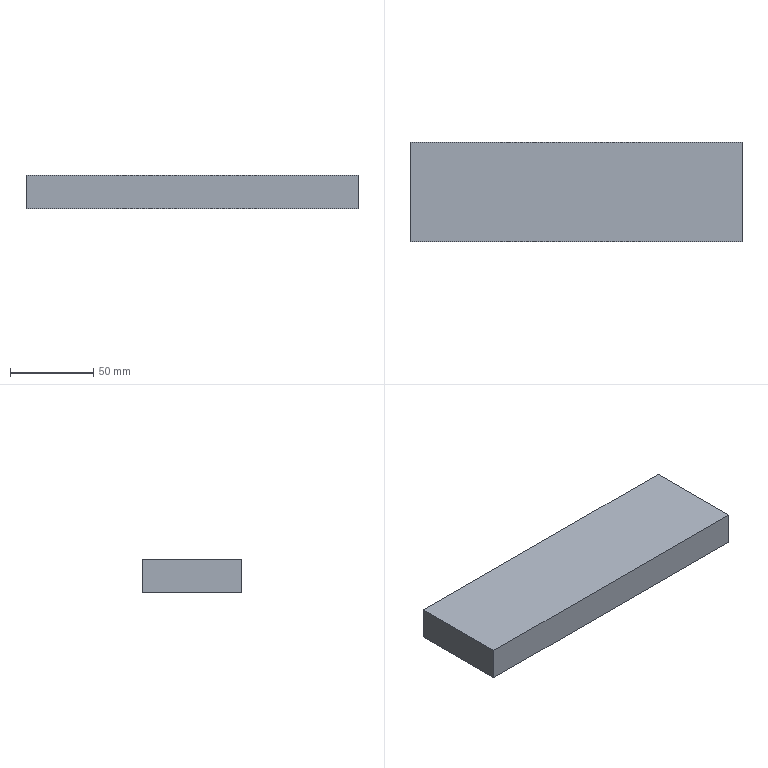Part | SolidWorks | features Extrusion 1 | 1 solid | 6 faces | box 200 x 60 x 20 mm | volume 240000 mm3 | plane 6
STEP:
#1=CARTESIAN_POINT('',(0.,60.,0.));
#2=VERTEX_POINT('',#1);
#3=CARTESIAN_POINT('',(0.,0.,0.));
#4=VERTEX_POINT('',#3);
#5=CARTESIAN_POINT('',(0.,0.,0.));
#6=DIRECTION('',(0.,-1.,0.));
#7=VECTOR('',#6,1000.);
#8=LINE('',#5,#7);
#9=EDGE_CURVE('',#2,#4,#8,.T.);
#10=ORIENTED_EDGE('',*,*,#9,.T.);
#11=CARTESIAN_POINT('',(0.,0.,20.));
#12=VERTEX_POINT('',#11);
#13=CARTESIAN_POINT('',(0.,0.,20.));
#14=DIRECTION('',(0.,0.,-1.));
#15=VECTOR('',#14,1000.);
#16=LINE('',#13,#15);
#17=EDGE_CURVE('',#12,#4,#16,.T.);
#18=ORIENTED_EDGE('',*,*,#17,.F.);
#19=CARTESIAN_POINT('',(0.,60.,20.));
#20=VERTEX_POINT('',#19);
#21=CARTESIAN_POINT('',(0.,0.,20.));
#22=DIRECTION('',(0.,-1.,0.));
#23=VECTOR('',#22,1000.);
#24=LINE('',#21,#23);
#25=EDGE_CURVE('',#20,#12,#24,.T.);
#26=ORIENTED_EDGE('',*,*,#25,.F.);
#27=CARTESIAN_POINT('',(0.,60.,20.));
#28=DIRECTION('',(0.,0.,-1.));
#29=VECTOR('',#28,1000.);
#30=LINE('',#27,#29);
#31=EDGE_CURVE('',#20,#2,#30,.T.);
#32=ORIENTED_EDGE('',*,*,#31,.T.);
#33=EDGE_LOOP('',(#10,#18,#26,#32));
#34=FACE_OUTER_BOUND('',#33,.T.);
#35=CARTESIAN_POINT('',(0.,0.,20.));
#36=DIRECTION('',(1.,0.,0.));
#37=DIRECTION('',(0.,0.,-1.));
#38=AXIS2_PLACEMENT_3D('',#35,#36,#37);
#39=PLANE('',#38);
#40=ADVANCED_FACE('',(#34),#39,.F.);
#41=CARTESIAN_POINT('',(200.,0.,0.));
#42=VERTEX_POINT('',#41);
#43=CARTESIAN_POINT('',(0.,0.,0.));
#44=DIRECTION('',(1.,0.,0.));
#45=VECTOR('',#44,1000.);
#46=LINE('',#43,#45);
#47=EDGE_CURVE('',#4,#42,#46,.T.);
#48=ORIENTED_EDGE('',*,*,#47,.T.);
#49=CARTESIAN_POINT('',(200.,0.,20.));
#50=VERTEX_POINT('',#49);
#51=CARTESIAN_POINT('',(200.,0.,20.));
#52=DIRECTION('',(0.,0.,-1.));
#53=VECTOR('',#52,1000.);
#54=LINE('',#51,#53);
#55=EDGE_CURVE('',#50,#42,#54,.T.);
#56=ORIENTED_EDGE('',*,*,#55,.F.);
#57=CARTESIAN_POINT('',(0.,0.,20.));
#58=DIRECTION('',(1.,0.,0.));
#59=VECTOR('',#58,1000.);
#60=LINE('',#57,#59);
#61=EDGE_CURVE('',#12,#50,#60,.T.);
#62=ORIENTED_EDGE('',*,*,#61,.F.);
#63=ORIENTED_EDGE('',*,*,#17,.T.);
#64=EDGE_LOOP('',(#48,#56,#62,#63));
#65=FACE_OUTER_BOUND('',#64,.T.);
#66=CARTESIAN_POINT('',(0.,0.,20.));
#67=DIRECTION('',(0.,1.,0.));
#68=DIRECTION('',(0.,0.,1.));
#69=AXIS2_PLACEMENT_3D('',#66,#67,#68);
#70=PLANE('',#69);
#71=ADVANCED_FACE('',(#65),#70,.F.);
#72=CARTESIAN_POINT('',(200.,60.,0.));
#73=VERTEX_POINT('',#72);
#74=CARTESIAN_POINT('',(200.,0.,0.));
#75=DIRECTION('',(0.,1.,0.));
#76=VECTOR('',#75,1000.);
#77=LINE('',#74,#76);
#78=EDGE_CURVE('',#42,#73,#77,.T.);
#79=ORIENTED_EDGE('',*,*,#78,.T.);
#80=CARTESIAN_POINT('',(200.,60.,20.));
#81=VERTEX_POINT('',#80);
#82=CARTESIAN_POINT('',(200.,60.,20.));
#83=DIRECTION('',(0.,0.,-1.));
#84=VECTOR('',#83,1000.);
#85=LINE('',#82,#84);
#86=EDGE_CURVE('',#81,#73,#85,.T.);
#87=ORIENTED_EDGE('',*,*,#86,.F.);
#88=CARTESIAN_POINT('',(200.,0.,20.));
#89=DIRECTION('',(0.,1.,0.));
#90=VECTOR('',#89,1000.);
#91=LINE('',#88,#90);
#92=EDGE_CURVE('',#50,#81,#91,.T.);
#93=ORIENTED_EDGE('',*,*,#92,.F.);
#94=ORIENTED_EDGE('',*,*,#55,.T.);
#95=EDGE_LOOP('',(#79,#87,#93,#94));
#96=FACE_OUTER_BOUND('',#95,.T.);
#97=CARTESIAN_POINT('',(200.,0.,20.));
#98=DIRECTION('',(-1.,0.,0.));
#99=DIRECTION('',(0.,0.,1.));
#100=AXIS2_PLACEMENT_3D('',#97,#98,#99);
#101=PLANE('',#100);
#102=ADVANCED_FACE('',(#96),#101,.F.);
#103=CARTESIAN_POINT('',(0.,60.,0.));
#104=DIRECTION('',(-1.,0.,0.));
#105=VECTOR('',#104,1000.);
#106=LINE('',#103,#105);
#107=EDGE_CURVE('',#73,#2,#106,.T.);
#108=ORIENTED_EDGE('',*,*,#107,.T.);
#109=ORIENTED_EDGE('',*,*,#31,.F.);
#110=CARTESIAN_POINT('',(0.,60.,20.));
#111=DIRECTION('',(-1.,0.,0.));
#112=VECTOR('',#111,1000.);
#113=LINE('',#110,#112);
#114=EDGE_CURVE('',#81,#20,#113,.T.);
#115=ORIENTED_EDGE('',*,*,#114,.F.);
#116=ORIENTED_EDGE('',*,*,#86,.T.);
#117=EDGE_LOOP('',(#108,#109,#115,#116));
#118=FACE_OUTER_BOUND('',#117,.T.);
#119=CARTESIAN_POINT('',(0.,60.,20.));
#120=DIRECTION('',(0.,-1.,0.));
#121=DIRECTION('',(0.,0.,-1.));
#122=AXIS2_PLACEMENT_3D('',#119,#120,#121);
#123=PLANE('',#122);
#124=ADVANCED_FACE('',(#118),#123,.F.);
#125=ORIENTED_EDGE('',*,*,#25,.T.);
#126=ORIENTED_EDGE('',*,*,#61,.T.);
#127=ORIENTED_EDGE('',*,*,#92,.T.);
#128=ORIENTED_EDGE('',*,*,#114,.T.);
#129=EDGE_LOOP('',(#125,#126,#127,#128));
#130=FACE_OUTER_BOUND('',#129,.T.);
#131=CARTESIAN_POINT('',(0.,0.,20.));
#132=DIRECTION('',(0.,0.,-1.));
#133=DIRECTION('',(-1.,0.,0.));
#134=AXIS2_PLACEMENT_3D('',#131,#132,#133);
#135=PLANE('',#134);
#136=ADVANCED_FACE('',(#130),#135,.F.);
#137=ORIENTED_EDGE('',*,*,#9,.F.);
#138=ORIENTED_EDGE('',*,*,#107,.F.);
#139=ORIENTED_EDGE('',*,*,#78,.F.);
#140=ORIENTED_EDGE('',*,*,#47,.F.);
#141=EDGE_LOOP('',(#137,#138,#139,#140));
#142=FACE_OUTER_BOUND('',#141,.T.);
#143=CARTESIAN_POINT('',(0.,0.,0.));
#144=DIRECTION('',(0.,0.,-1.));
#145=DIRECTION('',(-1.,0.,0.));
#146=AXIS2_PLACEMENT_3D('',#143,#144,#145);
#147=PLANE('',#146);
#148=ADVANCED_FACE('',(#142),#147,.T.);
#149=CLOSED_SHELL('',(#40,#71,#102,#124,#136,#148));
#150=MANIFOLD_SOLID_BREP('',#149);
#151=CARTESIAN_POINT('',(0.,0.,0.));
#152=DIRECTION('',(0.,0.,1.));
#153=DIRECTION('',(1.,0.,0.));
#154=AXIS2_PLACEMENT_3D('',#151,#152,#153);
#155=(LENGTH_UNIT()NAMED_UNIT(*)SI_UNIT(.MILLI.,.METRE.));
#156=UNCERTAINTY_MEASURE_WITH_UNIT(LENGTH_MEASURE(0.00001),#155,'','');
#157=(NAMED_UNIT(*)PLANE_ANGLE_UNIT()SI_UNIT($,.RADIAN.));
#158=(NAMED_UNIT(*)SI_UNIT($,.STERADIAN.)SOLID_ANGLE_UNIT());
#159=(GEOMETRIC_REPRESENTATION_CONTEXT(3)GLOBAL_UNCERTAINTY_ASSIGNED_CONTEXT((#156))GLOBAL_UNIT_ASSIGNED_CONTEXT((#155,#157,#158))REPRESENTATION_CONTEXT('',''));
#160=ADVANCED_BREP_SHAPE_REPRESENTATION('',(#150,#154),#159);